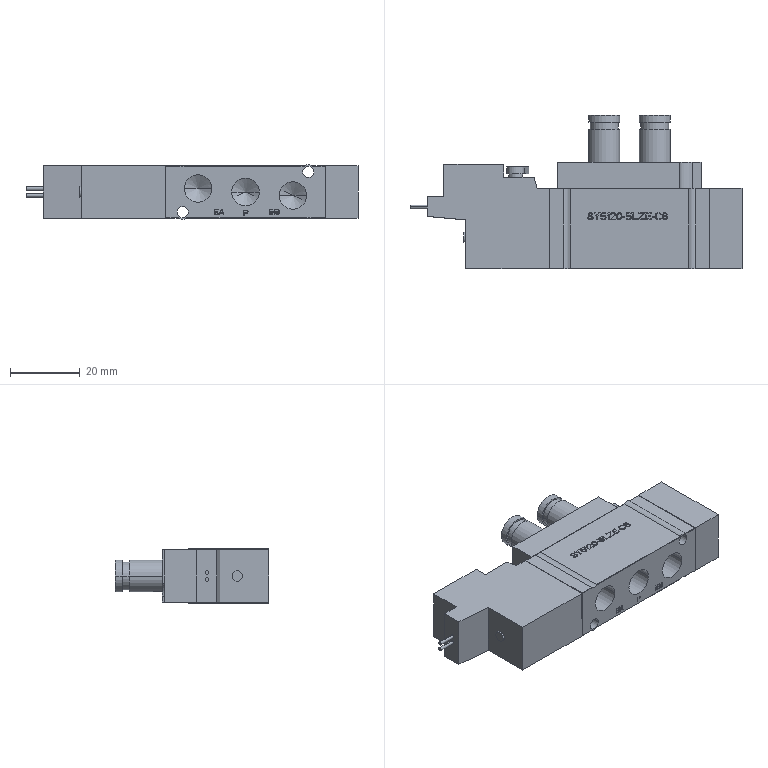Part | NX | 1 solid | 605 faces | box 95.3 x 44 x 15.6 mm | volume 33702 mm3 | plane 556 | cylinder 43 | cone 6 | commonest cylinder face diameters 9 x8 4 x6 7.938 x6 1 x4 3.2 x4 6 x4